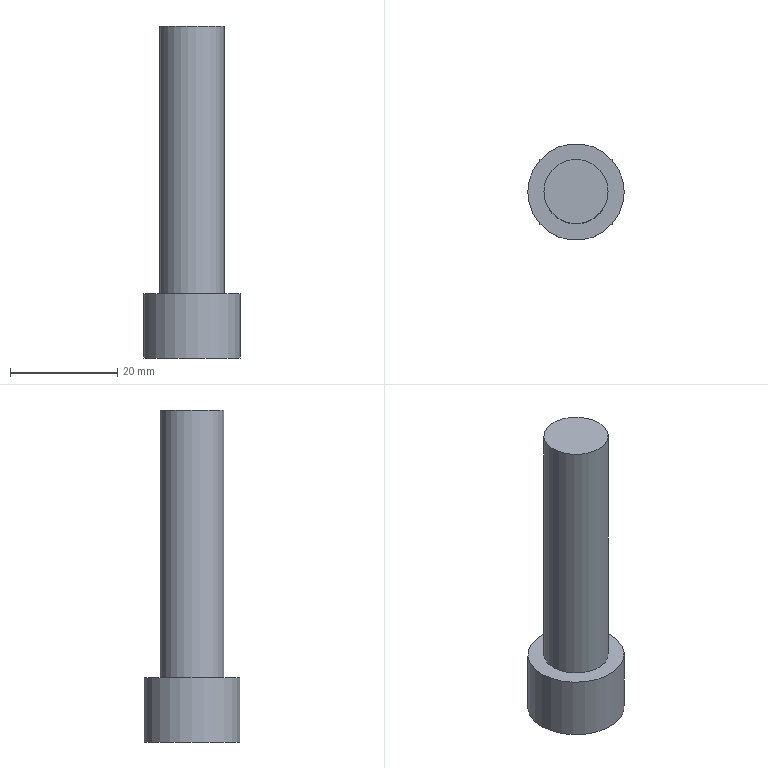Part | NX | features MAIN_BODY 2 | 1 solid | 5 faces | box 18 x 18 x 62 mm | volume 8708 mm3 | plane 3 | cylinder 2 | commonest cylinder face diameters 12 x1 18 x1
STEP:
#1=CARTESIAN_POINT('',(-481.5,210.,375.));
#2=VERTEX_POINT('',#1);
#3=CARTESIAN_POINT('',(-472.5,210.,375.));
#4=DIRECTION('',(0.,0.,-1.));
#5=DIRECTION('',(-1.,0.,0.));
#6=AXIS2_PLACEMENT_3D('',#3,#4,#5);
#7=CIRCLE('',#6,9.);
#8=EDGE_CURVE('',#2,#2,#7,.T.);
#9=ORIENTED_EDGE('',*,*,#8,.T.);
#10=EDGE_LOOP('',(#9));
#11=FACE_BOUND('',#10,.T.);
#12=CARTESIAN_POINT('',(-481.5,210.,363.));
#13=VERTEX_POINT('',#12);
#14=CARTESIAN_POINT('',(-472.5,210.,363.));
#15=DIRECTION('',(0.,0.,-1.));
#16=DIRECTION('',(-1.,0.,0.));
#17=AXIS2_PLACEMENT_3D('',#14,#15,#16);
#18=CIRCLE('',#17,9.);
#19=EDGE_CURVE('',#13,#13,#18,.T.);
#20=ORIENTED_EDGE('',*,*,#19,.F.);
#21=EDGE_LOOP('',(#20));
#22=FACE_BOUND('',#21,.T.);
#23=CARTESIAN_POINT('',(-472.5,210.,375.));
#24=DIRECTION('',(0.,0.,-1.));
#25=DIRECTION('',(-1.,0.,0.));
#26=AXIS2_PLACEMENT_3D('',#23,#24,#25);
#27=CYLINDRICAL_SURFACE('',#26,9.);
#28=ADVANCED_FACE('',(#11,#22),#27,.T.);
#29=CARTESIAN_POINT('',(-478.5,210.,375.));
#30=VERTEX_POINT('',#29);
#31=CARTESIAN_POINT('',(-472.5,210.,375.));
#32=DIRECTION('',(0.,0.,-1.));
#33=DIRECTION('',(-1.,0.,0.));
#34=AXIS2_PLACEMENT_3D('',#31,#32,#33);
#35=CIRCLE('',#34,6.);
#36=EDGE_CURVE('',#30,#30,#35,.T.);
#37=ORIENTED_EDGE('',*,*,#36,.T.);
#38=EDGE_LOOP('',(#37));
#39=FACE_BOUND('',#38,.T.);
#40=ORIENTED_EDGE('',*,*,#8,.F.);
#41=EDGE_LOOP('',(#40));
#42=FACE_BOUND('',#41,.T.);
#43=CARTESIAN_POINT('',(-472.5,210.,375.));
#44=DIRECTION('',(0.,0.,1.));
#45=DIRECTION('',(1.,0.,0.));
#46=AXIS2_PLACEMENT_3D('',#43,#44,#45);
#47=PLANE('',#46);
#48=ADVANCED_FACE('',(#39,#42),#47,.T.);
#49=ORIENTED_EDGE('',*,*,#19,.T.);
#50=EDGE_LOOP('',(#49));
#51=FACE_BOUND('',#50,.T.);
#52=CARTESIAN_POINT('',(-472.5,210.,363.));
#53=DIRECTION('',(0.,0.,1.));
#54=DIRECTION('',(1.,0.,0.));
#55=AXIS2_PLACEMENT_3D('',#52,#53,#54);
#56=PLANE('',#55);
#57=ADVANCED_FACE('',(#51),#56,.F.);
#58=CARTESIAN_POINT('',(-478.5,210.,425.));
#59=VERTEX_POINT('',#58);
#60=CARTESIAN_POINT('',(-472.5,210.,425.));
#61=DIRECTION('',(0.,0.,-1.));
#62=DIRECTION('',(-1.,0.,0.));
#63=AXIS2_PLACEMENT_3D('',#60,#61,#62);
#64=CIRCLE('',#63,6.);
#65=EDGE_CURVE('',#59,#59,#64,.F.);
#66=ORIENTED_EDGE('',*,*,#65,.T.);
#67=EDGE_LOOP('',(#66));
#68=FACE_BOUND('',#67,.T.);
#69=CARTESIAN_POINT('',(-472.5,210.,425.));
#70=DIRECTION('',(0.,0.,1.));
#71=DIRECTION('',(1.,0.,0.));
#72=AXIS2_PLACEMENT_3D('',#69,#70,#71);
#73=PLANE('',#72);
#74=ADVANCED_FACE('',(#68),#73,.T.);
#75=ORIENTED_EDGE('',*,*,#65,.F.);
#76=EDGE_LOOP('',(#75));
#77=FACE_BOUND('',#76,.T.);
#78=ORIENTED_EDGE('',*,*,#36,.F.);
#79=EDGE_LOOP('',(#78));
#80=FACE_BOUND('',#79,.T.);
#81=CARTESIAN_POINT('',(-472.5,210.,375.));
#82=DIRECTION('',(0.,0.,1.));
#83=DIRECTION('',(1.,0.,0.));
#84=AXIS2_PLACEMENT_3D('',#81,#82,#83);
#85=CYLINDRICAL_SURFACE('',#84,6.);
#86=ADVANCED_FACE('',(#77,#80),#85,.T.);
#87=CLOSED_SHELL('',(#28,#48,#57,#74,#86));
#88=MANIFOLD_SOLID_BREP('',#87);
#89=(LENGTH_UNIT()NAMED_UNIT(*)SI_UNIT(.MILLI.,.METRE.));
#90=UNCERTAINTY_MEASURE_WITH_UNIT(LENGTH_MEASURE(0.00001),#89,'','');
#91=(NAMED_UNIT(*)PLANE_ANGLE_UNIT()SI_UNIT($,.RADIAN.));
#92=(NAMED_UNIT(*)SI_UNIT($,.STERADIAN.)SOLID_ANGLE_UNIT());
#93=(GEOMETRIC_REPRESENTATION_CONTEXT(3)GLOBAL_UNCERTAINTY_ASSIGNED_CONTEXT((#90))GLOBAL_UNIT_ASSIGNED_CONTEXT((#89,#91,#92))REPRESENTATION_CONTEXT('',''));
#94=ADVANCED_BREP_SHAPE_REPRESENTATION('',(#88),#93);